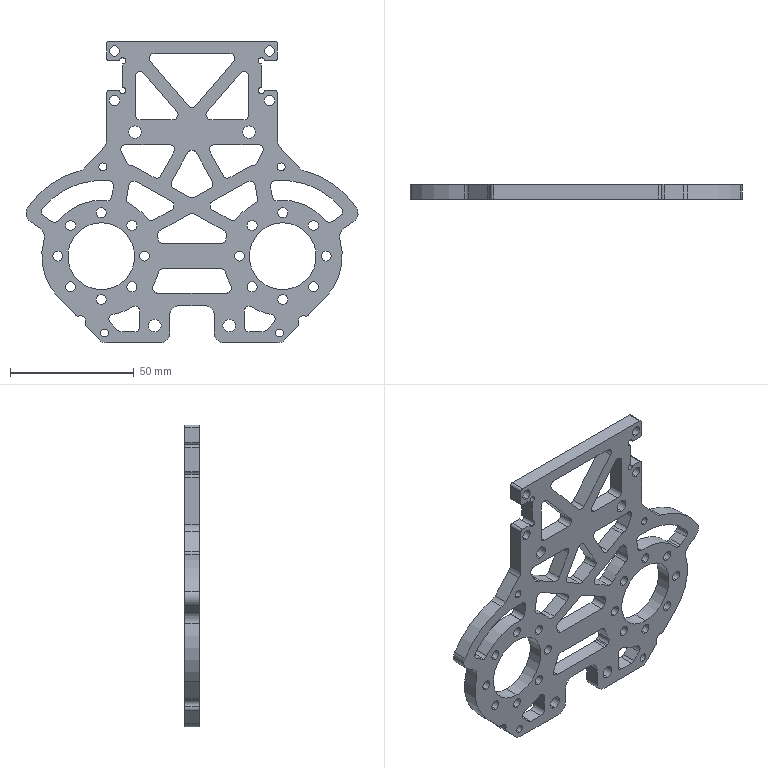Part | SolidWorks | features Fillet 3, ICE 2, Extrusion 1 | 1 solid | 248 faces | box 133.928 x 6 x 121.75 mm | volume 39124 mm3 | cylinder 178 | plane 70 | commonest cylinder face diameters 4 x68 4.02 x32 8 x14 48 x10 3.2 x8 4.2 x8